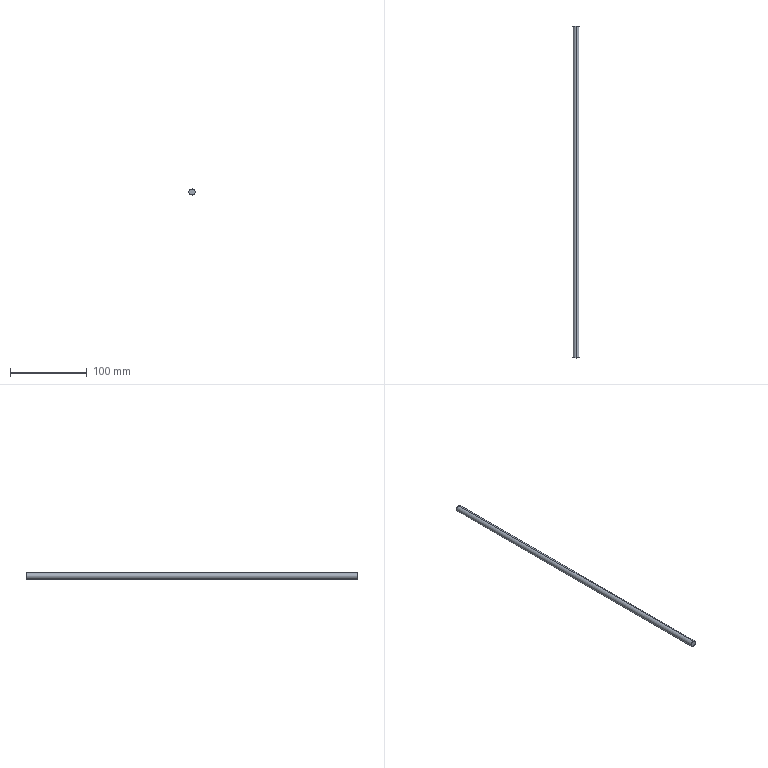Part | 1 solid | 4 faces | box 8 x 432 x 8 mm | volume 21715 mm3 | cylinder 2 | plane 2 | commonest cylinder face diameters 8 x2
STEP:
#1=CARTESIAN_POINT('',(0.,0.,0.));
#2=DIRECTION('',(0.,0.,1.));
#3=DIRECTION('',(1.,0.,0.));
#4=AXIS2_PLACEMENT_3D('',#1,#2,#3);
#5=CARTESIAN_POINT('',(-523.931,244.551,-285.55));
#6=VERTEX_POINT('',#5);
#7=CARTESIAN_POINT('',(-523.931,676.551,-285.55));
#8=VERTEX_POINT('',#7);
#9=CARTESIAN_POINT('',(-523.931,244.551,-285.55));
#10=DIRECTION('',(0.,1.,0.));
#11=VECTOR('',#10,1.);
#12=LINE('',#9,#11);
#13=CARTESIAN_POINT('',(-523.931,61.551,-281.55));
#14=DIRECTION('',(0.,1.,0.));
#15=DIRECTION('',(1.,0.,0.));
#16=AXIS2_PLACEMENT_3D('',#13,#14,#15);
#17=CYLINDRICAL_SURFACE('',#16,4.);
#18=CARTESIAN_POINT('',(1.571,183.));
#19=DIRECTION('',(0.,1.));
#20=VECTOR('',#19,1.);
#21=LINE('',#18,#20);
#22=(GEOMETRIC_REPRESENTATION_CONTEXT(2)PARAMETRIC_REPRESENTATION_CONTEXT()REPRESENTATION_CONTEXT('',''));
#23=DEFINITIONAL_REPRESENTATION('',(#21),#22);
#24=PCURVE('',#17,#23);
#25=CARTESIAN_POINT('',(-523.931,61.551,-281.55));
#26=DIRECTION('',(0.,1.,0.));
#27=DIRECTION('',(-1.,0.,0.));
#28=AXIS2_PLACEMENT_3D('',#25,#26,#27);
#29=CYLINDRICAL_SURFACE('',#28,4.);
#30=CARTESIAN_POINT('',(4.712,183.));
#31=DIRECTION('',(0.,1.));
#32=VECTOR('',#31,1.);
#33=LINE('',#30,#32);
#34=(GEOMETRIC_REPRESENTATION_CONTEXT(2)PARAMETRIC_REPRESENTATION_CONTEXT()REPRESENTATION_CONTEXT('',''));
#35=DEFINITIONAL_REPRESENTATION('',(#33),#34);
#36=PCURVE('',#29,#35);
#37=SURFACE_CURVE('',#12,(#24,#36),.PCURVE_S1.);
#38=EDGE_CURVE('',#6,#8,#37,.T.);
#39=ORIENTED_EDGE('',*,*,#38,.F.);
#40=CARTESIAN_POINT('',(-523.931,244.551,-277.55));
#41=VERTEX_POINT('',#40);
#42=CARTESIAN_POINT('',(-523.931,244.551,-281.55));
#43=DIRECTION('',(0.,-1.,0.));
#44=DIRECTION('',(0.,0.,1.));
#45=AXIS2_PLACEMENT_3D('',#42,#43,#44);
#46=CIRCLE('',#45,4.);
#47=CARTESIAN_POINT('',(4.712,183.));
#48=DIRECTION('',(-1.,0.));
#49=VECTOR('',#48,1.);
#50=LINE('',#47,#49);
#51=(GEOMETRIC_REPRESENTATION_CONTEXT(2)PARAMETRIC_REPRESENTATION_CONTEXT()REPRESENTATION_CONTEXT('',''));
#52=DEFINITIONAL_REPRESENTATION('',(#50),#51);
#53=PCURVE('',#17,#52);
#54=CARTESIAN_POINT('',(-523.931,244.551,-281.55));
#55=DIRECTION('',(0.,-1.,0.));
#56=DIRECTION('',(0.,0.,-1.));
#57=AXIS2_PLACEMENT_3D('',#54,#55,#56);
#58=PLANE('',#57);
#59=CARTESIAN_POINT('',(0.,0.));
#60=DIRECTION('',(-1.,0.));
#61=AXIS2_PLACEMENT_2D('',#59,#60);
#62=CIRCLE('',#61,4.);
#63=(GEOMETRIC_REPRESENTATION_CONTEXT(2)PARAMETRIC_REPRESENTATION_CONTEXT()REPRESENTATION_CONTEXT('',''));
#64=DEFINITIONAL_REPRESENTATION('',(#62),#63);
#65=PCURVE('',#58,#64);
#66=SURFACE_CURVE('',#46,(#53,#65),.PCURVE_S1.);
#67=EDGE_CURVE('',#41,#6,#66,.T.);
#68=ORIENTED_EDGE('',*,*,#67,.F.);
#69=CARTESIAN_POINT('',(-523.931,676.551,-277.55));
#70=VERTEX_POINT('',#69);
#71=CARTESIAN_POINT('',(-523.931,244.551,-277.55));
#72=DIRECTION('',(0.,1.,0.));
#73=VECTOR('',#72,1.);
#74=LINE('',#71,#73);
#75=CARTESIAN_POINT('',(4.712,183.));
#76=DIRECTION('',(0.,1.));
#77=VECTOR('',#76,1.);
#78=LINE('',#75,#77);
#79=(GEOMETRIC_REPRESENTATION_CONTEXT(2)PARAMETRIC_REPRESENTATION_CONTEXT()REPRESENTATION_CONTEXT('',''));
#80=DEFINITIONAL_REPRESENTATION('',(#78),#79);
#81=PCURVE('',#17,#80);
#82=CARTESIAN_POINT('',(1.571,183.));
#83=DIRECTION('',(0.,1.));
#84=VECTOR('',#83,1.);
#85=LINE('',#82,#84);
#86=(GEOMETRIC_REPRESENTATION_CONTEXT(2)PARAMETRIC_REPRESENTATION_CONTEXT()REPRESENTATION_CONTEXT('',''));
#87=DEFINITIONAL_REPRESENTATION('',(#85),#86);
#88=PCURVE('',#29,#87);
#89=SURFACE_CURVE('',#74,(#81,#88),.PCURVE_S1.);
#90=EDGE_CURVE('',#41,#70,#89,.T.);
#91=ORIENTED_EDGE('',*,*,#90,.T.);
#92=CARTESIAN_POINT('',(-523.931,676.551,-281.55));
#93=DIRECTION('',(0.,-1.,0.));
#94=DIRECTION('',(0.,0.,1.));
#95=AXIS2_PLACEMENT_3D('',#92,#93,#94);
#96=CIRCLE('',#95,4.);
#97=CARTESIAN_POINT('',(4.712,615.));
#98=DIRECTION('',(-1.,0.));
#99=VECTOR('',#98,1.);
#100=LINE('',#97,#99);
#101=(GEOMETRIC_REPRESENTATION_CONTEXT(2)PARAMETRIC_REPRESENTATION_CONTEXT()REPRESENTATION_CONTEXT('',''));
#102=DEFINITIONAL_REPRESENTATION('',(#100),#101);
#103=PCURVE('',#17,#102);
#104=CARTESIAN_POINT('',(-523.931,676.551,-281.55));
#105=DIRECTION('',(0.,-1.,0.));
#106=DIRECTION('',(0.,0.,-1.));
#107=AXIS2_PLACEMENT_3D('',#104,#105,#106);
#108=PLANE('',#107);
#109=CARTESIAN_POINT('',(0.,0.));
#110=DIRECTION('',(-1.,0.));
#111=AXIS2_PLACEMENT_2D('',#109,#110);
#112=CIRCLE('',#111,4.);
#113=(GEOMETRIC_REPRESENTATION_CONTEXT(2)PARAMETRIC_REPRESENTATION_CONTEXT()REPRESENTATION_CONTEXT('',''));
#114=DEFINITIONAL_REPRESENTATION('',(#112),#113);
#115=PCURVE('',#108,#114);
#116=SURFACE_CURVE('',#96,(#103,#115),.PCURVE_S1.);
#117=EDGE_CURVE('',#70,#8,#116,.T.);
#118=ORIENTED_EDGE('',*,*,#117,.T.);
#119=EDGE_LOOP('',(#39,#68,#91,#118));
#120=FACE_BOUND('',#119,.T.);
#121=ADVANCED_FACE('',(#120),#17,.T.);
#122=ORIENTED_EDGE('',*,*,#67,.T.);
#123=CARTESIAN_POINT('',(-523.931,244.551,-281.55));
#124=DIRECTION('',(0.,-1.,0.));
#125=DIRECTION('',(0.,0.,1.));
#126=AXIS2_PLACEMENT_3D('',#123,#124,#125);
#127=CIRCLE('',#126,4.);
#128=CARTESIAN_POINT('',(0.,0.));
#129=DIRECTION('',(-1.,0.));
#130=AXIS2_PLACEMENT_2D('',#128,#129);
#131=CIRCLE('',#130,4.);
#132=(GEOMETRIC_REPRESENTATION_CONTEXT(2)PARAMETRIC_REPRESENTATION_CONTEXT()REPRESENTATION_CONTEXT('',''));
#133=DEFINITIONAL_REPRESENTATION('',(#131),#132);
#134=PCURVE('',#58,#133);
#135=CARTESIAN_POINT('',(7.854,183.));
#136=DIRECTION('',(-1.,0.));
#137=VECTOR('',#136,1.);
#138=LINE('',#135,#137);
#139=(GEOMETRIC_REPRESENTATION_CONTEXT(2)PARAMETRIC_REPRESENTATION_CONTEXT()REPRESENTATION_CONTEXT('',''));
#140=DEFINITIONAL_REPRESENTATION('',(#138),#139);
#141=PCURVE('',#29,#140);
#142=SURFACE_CURVE('',#127,(#134,#141),.PCURVE_S1.);
#143=EDGE_CURVE('',#6,#41,#142,.T.);
#144=ORIENTED_EDGE('',*,*,#143,.T.);
#145=EDGE_LOOP('',(#122,#144));
#146=FACE_BOUND('',#145,.T.);
#147=ADVANCED_FACE('',(#146),#58,.T.);
#148=CARTESIAN_POINT('',(-523.931,676.551,-281.55));
#149=DIRECTION('',(0.,-1.,0.));
#150=DIRECTION('',(0.,0.,1.));
#151=AXIS2_PLACEMENT_3D('',#148,#149,#150);
#152=CIRCLE('',#151,4.);
#153=CARTESIAN_POINT('',(0.,0.));
#154=DIRECTION('',(-1.,0.));
#155=AXIS2_PLACEMENT_2D('',#153,#154);
#156=CIRCLE('',#155,4.);
#157=(GEOMETRIC_REPRESENTATION_CONTEXT(2)PARAMETRIC_REPRESENTATION_CONTEXT()REPRESENTATION_CONTEXT('',''));
#158=DEFINITIONAL_REPRESENTATION('',(#156),#157);
#159=PCURVE('',#108,#158);
#160=CARTESIAN_POINT('',(7.854,615.));
#161=DIRECTION('',(-1.,0.));
#162=VECTOR('',#161,1.);
#163=LINE('',#160,#162);
#164=(GEOMETRIC_REPRESENTATION_CONTEXT(2)PARAMETRIC_REPRESENTATION_CONTEXT()REPRESENTATION_CONTEXT('',''));
#165=DEFINITIONAL_REPRESENTATION('',(#163),#164);
#166=PCURVE('',#29,#165);
#167=SURFACE_CURVE('',#152,(#159,#166),.PCURVE_S1.);
#168=EDGE_CURVE('',#8,#70,#167,.T.);
#169=ORIENTED_EDGE('',*,*,#168,.F.);
#170=ORIENTED_EDGE('',*,*,#117,.F.);
#171=EDGE_LOOP('',(#169,#170));
#172=FACE_BOUND('',#171,.T.);
#173=ADVANCED_FACE('',(#172),#108,.F.);
#174=ORIENTED_EDGE('',*,*,#38,.T.);
#175=ORIENTED_EDGE('',*,*,#168,.T.);
#176=ORIENTED_EDGE('',*,*,#90,.F.);
#177=ORIENTED_EDGE('',*,*,#143,.F.);
#178=EDGE_LOOP('',(#174,#175,#176,#177));
#179=FACE_BOUND('',#178,.T.);
#180=ADVANCED_FACE('',(#179),#29,.T.);
#181=CLOSED_SHELL('',(#121,#147,#173,#180));
#182=MANIFOLD_SOLID_BREP('',#181);
#183=(LENGTH_UNIT()NAMED_UNIT(*)SI_UNIT(.MILLI.,.METRE.));
#184=UNCERTAINTY_MEASURE_WITH_UNIT(LENGTH_MEASURE(0.0000001),#183,'','');
#185=(NAMED_UNIT(*)PLANE_ANGLE_UNIT()SI_UNIT($,.RADIAN.));
#186=(NAMED_UNIT(*)SI_UNIT($,.STERADIAN.)SOLID_ANGLE_UNIT());
#187=(GEOMETRIC_REPRESENTATION_CONTEXT(3)GLOBAL_UNCERTAINTY_ASSIGNED_CONTEXT((#184))GLOBAL_UNIT_ASSIGNED_CONTEXT((#183,#185,#186))REPRESENTATION_CONTEXT('',''));
#188=ADVANCED_BREP_SHAPE_REPRESENTATION('',(#4,#182),#187);